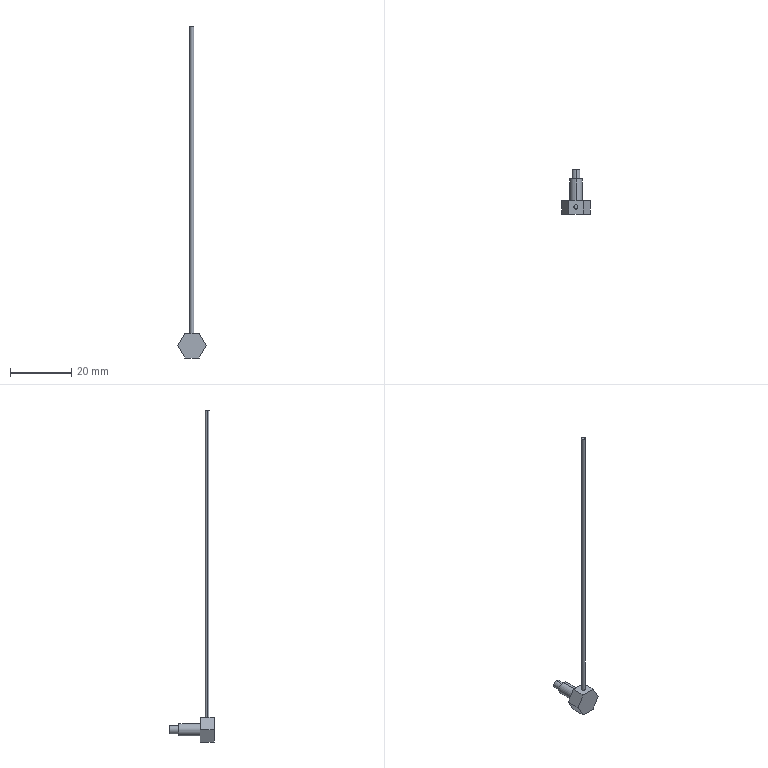Part | SolidWorks | features BaseBody 8 | 1 solid | 17 faces | box 9.238 x 14.5 x 108 mm | volume 486.04 mm3 | plane 11 | cylinder 6 | commonest cylinder face diameters 1.3 x2 2.6 x2 4 x2
STEP:
#1=CARTESIAN_POINT('',(-0.66,0.,100.));
#2=VERTEX_POINT('',#1);
#3=CARTESIAN_POINT('',(0.64,0.,100.));
#4=VERTEX_POINT('',#3);
#5=CARTESIAN_POINT('',(-0.01,0.,100.));
#6=DIRECTION('',(0.,0.,-1.));
#7=DIRECTION('',(-1.,0.,0.));
#8=AXIS2_PLACEMENT_3D('',#5,#6,#7);
#9=CIRCLE('',#8,0.65);
#10=EDGE_CURVE('',#2,#4,#9,.T.);
#11=ORIENTED_EDGE('',*,*,#10,.T.);
#12=CARTESIAN_POINT('',(0.64,0.,0.));
#13=VERTEX_POINT('',#12);
#14=CARTESIAN_POINT('',(0.64,0.,100.));
#15=DIRECTION('',(0.,0.,-1.));
#16=VECTOR('',#15,1000.);
#17=LINE('',#14,#16);
#18=EDGE_CURVE('',#4,#13,#17,.T.);
#19=ORIENTED_EDGE('',*,*,#18,.T.);
#20=CARTESIAN_POINT('',(-0.66,0.,0.));
#21=VERTEX_POINT('',#20);
#22=CARTESIAN_POINT('',(-0.01,0.,0.));
#23=DIRECTION('',(0.,0.,1.));
#24=DIRECTION('',(-1.,0.,0.));
#25=AXIS2_PLACEMENT_3D('',#22,#23,#24);
#26=CIRCLE('',#25,0.65);
#27=EDGE_CURVE('',#13,#21,#26,.T.);
#28=ORIENTED_EDGE('',*,*,#27,.T.);
#29=CARTESIAN_POINT('',(-0.66,0.,100.));
#30=DIRECTION('',(0.,0.,-1.));
#31=VECTOR('',#30,1000.);
#32=LINE('',#29,#31);
#33=EDGE_CURVE('',#2,#21,#32,.T.);
#34=ORIENTED_EDGE('',*,*,#33,.F.);
#35=EDGE_LOOP('',(#11,#19,#28,#34));
#36=FACE_OUTER_BOUND('',#35,.T.);
#37=CARTESIAN_POINT('',(-0.01,0.,100.));
#38=DIRECTION('',(0.,0.,-1.));
#39=DIRECTION('',(-1.,0.,0.));
#40=AXIS2_PLACEMENT_3D('',#37,#38,#39);
#41=CYLINDRICAL_SURFACE('',#40,0.65);
#42=ADVANCED_FACE('',(#36),#41,.T.);
#43=CARTESIAN_POINT('',(0.,9.25,-6.));
#44=VERTEX_POINT('',#43);
#45=CARTESIAN_POINT('',(0.,9.25,-2.));
#46=VERTEX_POINT('',#45);
#47=CARTESIAN_POINT('',(0.,9.25,-4.));
#48=DIRECTION('',(0.,-1.,0.));
#49=DIRECTION('',(0.,0.,-1.));
#50=AXIS2_PLACEMENT_3D('',#47,#48,#49);
#51=CIRCLE('',#50,2.);
#52=EDGE_CURVE('',#44,#46,#51,.T.);
#53=ORIENTED_EDGE('',*,*,#52,.T.);
#54=CARTESIAN_POINT('',(0.,2.25,-2.));
#55=VERTEX_POINT('',#54);
#56=CARTESIAN_POINT('',(0.,9.25,-2.));
#57=DIRECTION('',(0.,-1.,0.));
#58=VECTOR('',#57,1000.);
#59=LINE('',#56,#58);
#60=EDGE_CURVE('',#46,#55,#59,.T.);
#61=ORIENTED_EDGE('',*,*,#60,.T.);
#62=CARTESIAN_POINT('',(0.,2.25,-6.));
#63=VERTEX_POINT('',#62);
#64=CARTESIAN_POINT('',(0.,2.25,-4.));
#65=DIRECTION('',(0.,1.,0.));
#66=DIRECTION('',(0.,0.,-1.));
#67=AXIS2_PLACEMENT_3D('',#64,#65,#66);
#68=CIRCLE('',#67,2.);
#69=EDGE_CURVE('',#55,#63,#68,.T.);
#70=ORIENTED_EDGE('',*,*,#69,.T.);
#71=CARTESIAN_POINT('',(0.,9.25,-6.));
#72=DIRECTION('',(0.,-1.,0.));
#73=VECTOR('',#72,1000.);
#74=LINE('',#71,#73);
#75=EDGE_CURVE('',#44,#63,#74,.T.);
#76=ORIENTED_EDGE('',*,*,#75,.F.);
#77=EDGE_LOOP('',(#53,#61,#70,#76));
#78=FACE_OUTER_BOUND('',#77,.T.);
#79=CARTESIAN_POINT('',(0.,9.25,-4.));
#80=DIRECTION('',(0.,-1.,0.));
#81=DIRECTION('',(0.,0.,-1.));
#82=AXIS2_PLACEMENT_3D('',#79,#80,#81);
#83=CYLINDRICAL_SURFACE('',#82,2.);
#84=ADVANCED_FACE('',(#78),#83,.T.);
#85=CARTESIAN_POINT('',(0.,12.25,-5.3));
#86=VERTEX_POINT('',#85);
#87=CARTESIAN_POINT('',(0.,12.25,-2.7));
#88=VERTEX_POINT('',#87);
#89=CARTESIAN_POINT('',(0.,12.25,-4.));
#90=DIRECTION('',(0.,-1.,0.));
#91=DIRECTION('',(0.,0.,-1.));
#92=AXIS2_PLACEMENT_3D('',#89,#90,#91);
#93=CIRCLE('',#92,1.3);
#94=EDGE_CURVE('',#86,#88,#93,.T.);
#95=ORIENTED_EDGE('',*,*,#94,.T.);
#96=CARTESIAN_POINT('',(0.,9.25,-2.7));
#97=VERTEX_POINT('',#96);
#98=CARTESIAN_POINT('',(0.,12.25,-2.7));
#99=DIRECTION('',(0.,-1.,0.));
#100=VECTOR('',#99,1000.);
#101=LINE('',#98,#100);
#102=EDGE_CURVE('',#88,#97,#101,.T.);
#103=ORIENTED_EDGE('',*,*,#102,.T.);
#104=CARTESIAN_POINT('',(0.,9.25,-5.3));
#105=VERTEX_POINT('',#104);
#106=CARTESIAN_POINT('',(0.,9.25,-4.));
#107=DIRECTION('',(0.,-1.,0.));
#108=DIRECTION('',(0.,0.,-1.));
#109=AXIS2_PLACEMENT_3D('',#106,#107,#108);
#110=CIRCLE('',#109,1.3);
#111=EDGE_CURVE('',#105,#97,#110,.T.);
#112=ORIENTED_EDGE('',*,*,#111,.F.);
#113=CARTESIAN_POINT('',(0.,12.25,-5.3));
#114=DIRECTION('',(0.,-1.,0.));
#115=VECTOR('',#114,1000.);
#116=LINE('',#113,#115);
#117=EDGE_CURVE('',#86,#105,#116,.T.);
#118=ORIENTED_EDGE('',*,*,#117,.F.);
#119=EDGE_LOOP('',(#95,#103,#112,#118));
#120=FACE_OUTER_BOUND('',#119,.T.);
#121=CARTESIAN_POINT('',(0.,12.25,-4.));
#122=DIRECTION('',(0.,-1.,0.));
#123=DIRECTION('',(0.,0.,-1.));
#124=AXIS2_PLACEMENT_3D('',#121,#122,#123);
#125=CYLINDRICAL_SURFACE('',#124,1.3);
#126=ADVANCED_FACE('',(#120),#125,.T.);
#127=ORIENTED_EDGE('',*,*,#18,.F.);
#128=CARTESIAN_POINT('',(-0.01,0.,100.));
#129=DIRECTION('',(0.,0.,-1.));
#130=DIRECTION('',(-1.,0.,0.));
#131=AXIS2_PLACEMENT_3D('',#128,#129,#130);
#132=CIRCLE('',#131,0.65);
#133=EDGE_CURVE('',#4,#2,#132,.T.);
#134=ORIENTED_EDGE('',*,*,#133,.T.);
#135=ORIENTED_EDGE('',*,*,#33,.T.);
#136=CARTESIAN_POINT('',(-0.01,0.,0.));
#137=DIRECTION('',(0.,0.,1.));
#138=DIRECTION('',(-1.,0.,0.));
#139=AXIS2_PLACEMENT_3D('',#136,#137,#138);
#140=CIRCLE('',#139,0.65);
#141=EDGE_CURVE('',#21,#13,#140,.T.);
#142=ORIENTED_EDGE('',*,*,#141,.T.);
#143=EDGE_LOOP('',(#127,#134,#135,#142));
#144=FACE_OUTER_BOUND('',#143,.T.);
#145=CARTESIAN_POINT('',(-0.01,0.,100.));
#146=DIRECTION('',(0.,0.,-1.));
#147=DIRECTION('',(-1.,0.,0.));
#148=AXIS2_PLACEMENT_3D('',#145,#146,#147);
#149=CYLINDRICAL_SURFACE('',#148,0.65);
#150=ADVANCED_FACE('',(#144),#149,.T.);
#151=ORIENTED_EDGE('',*,*,#141,.F.);
#152=ORIENTED_EDGE('',*,*,#27,.F.);
#153=EDGE_LOOP('',(#151,#152));
#154=FACE_BOUND('',#153,.T.);
#155=CARTESIAN_POINT('',(-2.309,-2.25,0.));
#156=VERTEX_POINT('',#155);
#157=CARTESIAN_POINT('',(-2.309,2.25,0.));
#158=VERTEX_POINT('',#157);
#159=CARTESIAN_POINT('',(-2.309,-2.25,0.));
#160=DIRECTION('',(0.,1.,0.));
#161=VECTOR('',#160,1000.);
#162=LINE('',#159,#161);
#163=EDGE_CURVE('',#156,#158,#162,.T.);
#164=ORIENTED_EDGE('',*,*,#163,.F.);
#165=CARTESIAN_POINT('',(2.309,-2.25,0.));
#166=VERTEX_POINT('',#165);
#167=CARTESIAN_POINT('',(-2.309,-2.25,0.));
#168=DIRECTION('',(-1.,0.,0.));
#169=VECTOR('',#168,1000.);
#170=LINE('',#167,#169);
#171=EDGE_CURVE('',#166,#156,#170,.T.);
#172=ORIENTED_EDGE('',*,*,#171,.F.);
#173=CARTESIAN_POINT('',(2.309,2.25,0.));
#174=VERTEX_POINT('',#173);
#175=CARTESIAN_POINT('',(2.309,-2.25,0.));
#176=DIRECTION('',(0.,-1.,0.));
#177=VECTOR('',#176,1000.);
#178=LINE('',#175,#177);
#179=EDGE_CURVE('',#174,#166,#178,.T.);
#180=ORIENTED_EDGE('',*,*,#179,.F.);
#181=CARTESIAN_POINT('',(-2.309,2.25,0.));
#182=DIRECTION('',(1.,0.,0.));
#183=VECTOR('',#182,1000.);
#184=LINE('',#181,#183);
#185=EDGE_CURVE('',#158,#174,#184,.T.);
#186=ORIENTED_EDGE('',*,*,#185,.F.);
#187=EDGE_LOOP('',(#164,#172,#180,#186));
#188=FACE_OUTER_BOUND('',#187,.T.);
#189=CARTESIAN_POINT('',(-2.309,-2.25,0.));
#190=DIRECTION('',(0.,0.,-1.));
#191=DIRECTION('',(-1.,0.,0.));
#192=AXIS2_PLACEMENT_3D('',#189,#190,#191);
#193=PLANE('',#192);
#194=ADVANCED_FACE('',(#154,#188),#193,.F.);
#195=ORIENTED_EDGE('',*,*,#10,.F.);
#196=ORIENTED_EDGE('',*,*,#133,.F.);
#197=EDGE_LOOP('',(#195,#196));
#198=FACE_OUTER_BOUND('',#197,.T.);
#199=CARTESIAN_POINT('',(-0.01,0.,100.));
#200=DIRECTION('',(0.,0.,1.));
#201=DIRECTION('',(1.,0.,0.));
#202=AXIS2_PLACEMENT_3D('',#199,#200,#201);
#203=PLANE('',#202);
#204=ADVANCED_FACE('',(#198),#203,.T.);
#205=CARTESIAN_POINT('',(0.,2.25,-4.));
#206=DIRECTION('',(0.,1.,0.));
#207=DIRECTION('',(0.,0.,-1.));
#208=AXIS2_PLACEMENT_3D('',#205,#206,#207);
#209=CIRCLE('',#208,2.);
#210=EDGE_CURVE('',#63,#55,#209,.T.);
#211=ORIENTED_EDGE('',*,*,#210,.F.);
#212=ORIENTED_EDGE('',*,*,#69,.F.);
#213=EDGE_LOOP('',(#211,#212));
#214=FACE_BOUND('',#213,.T.);
#215=ORIENTED_EDGE('',*,*,#185,.T.);
#216=CARTESIAN_POINT('',(4.619,2.25,-4.));
#217=VERTEX_POINT('',#216);
#218=CARTESIAN_POINT('',(4.619,2.25,-4.));
#219=DIRECTION('',(-0.5,0.,0.866));
#220=VECTOR('',#219,1000.);
#221=LINE('',#218,#220);
#222=EDGE_CURVE('',#217,#174,#221,.T.);
#223=ORIENTED_EDGE('',*,*,#222,.F.);
#224=CARTESIAN_POINT('',(2.309,2.25,-8.));
#225=VERTEX_POINT('',#224);
#226=CARTESIAN_POINT('',(2.309,2.25,-8.));
#227=DIRECTION('',(0.5,0.,0.866));
#228=VECTOR('',#227,1000.);
#229=LINE('',#226,#228);
#230=EDGE_CURVE('',#225,#217,#229,.T.);
#231=ORIENTED_EDGE('',*,*,#230,.F.);
#232=CARTESIAN_POINT('',(-2.309,2.25,-8.));
#233=VERTEX_POINT('',#232);
#234=CARTESIAN_POINT('',(-2.309,2.25,-8.));
#235=DIRECTION('',(1.,0.,0.));
#236=VECTOR('',#235,1000.);
#237=LINE('',#234,#236);
#238=EDGE_CURVE('',#233,#225,#237,.T.);
#239=ORIENTED_EDGE('',*,*,#238,.F.);
#240=CARTESIAN_POINT('',(-4.619,2.25,-4.));
#241=VERTEX_POINT('',#240);
#242=CARTESIAN_POINT('',(-4.619,2.25,-4.));
#243=DIRECTION('',(0.5,0.,-0.866));
#244=VECTOR('',#243,1000.);
#245=LINE('',#242,#244);
#246=EDGE_CURVE('',#241,#233,#245,.T.);
#247=ORIENTED_EDGE('',*,*,#246,.F.);
#248=CARTESIAN_POINT('',(-2.309,2.25,0.));
#249=DIRECTION('',(-0.5,0.,-0.866));
#250=VECTOR('',#249,1000.);
#251=LINE('',#248,#250);
#252=EDGE_CURVE('',#158,#241,#251,.T.);
#253=ORIENTED_EDGE('',*,*,#252,.F.);
#254=EDGE_LOOP('',(#215,#223,#231,#239,#247,#253));
#255=FACE_OUTER_BOUND('',#254,.T.);
#256=CARTESIAN_POINT('',(-2.309,2.25,0.));
#257=DIRECTION('',(0.,-1.,0.));
#258=DIRECTION('',(0.,0.,-1.));
#259=AXIS2_PLACEMENT_3D('',#256,#257,#258);
#260=PLANE('',#259);
#261=ADVANCED_FACE('',(#214,#255),#260,.F.);
#262=CARTESIAN_POINT('',(-4.619,-2.25,-4.));
#263=VERTEX_POINT('',#262);
#264=CARTESIAN_POINT('',(-4.619,-2.25,-4.));
#265=DIRECTION('',(0.,1.,0.));
#266=VECTOR('',#265,1000.);
#267=LINE('',#264,#266);
#268=EDGE_CURVE('',#263,#241,#267,.T.);
#269=ORIENTED_EDGE('',*,*,#268,.F.);
#270=CARTESIAN_POINT('',(-4.619,-2.25,-4.));
#271=DIRECTION('',(-0.5,0.,-0.866));
#272=VECTOR('',#271,1000.);
#273=LINE('',#270,#272);
#274=EDGE_CURVE('',#156,#263,#273,.T.);
#275=ORIENTED_EDGE('',*,*,#274,.F.);
#276=ORIENTED_EDGE('',*,*,#163,.T.);
#277=ORIENTED_EDGE('',*,*,#252,.T.);
#278=EDGE_LOOP('',(#269,#275,#276,#277));
#279=FACE_OUTER_BOUND('',#278,.T.);
#280=CARTESIAN_POINT('',(-4.619,-2.25,-4.));
#281=DIRECTION('',(0.866,0.,-0.5));
#282=DIRECTION('',(-0.5,0.,-0.866));
#283=AXIS2_PLACEMENT_3D('',#280,#281,#282);
#284=PLANE('',#283);
#285=ADVANCED_FACE('',(#279),#284,.F.);
#286=CARTESIAN_POINT('',(4.619,-2.25,-4.));
#287=VERTEX_POINT('',#286);
#288=CARTESIAN_POINT('',(4.619,-2.25,-4.));
#289=DIRECTION('',(-0.5,0.,0.866));
#290=VECTOR('',#289,1000.);
#291=LINE('',#288,#290);
#292=EDGE_CURVE('',#287,#166,#291,.T.);
#293=ORIENTED_EDGE('',*,*,#292,.T.);
#294=ORIENTED_EDGE('',*,*,#171,.T.);
#295=ORIENTED_EDGE('',*,*,#274,.T.);
#296=CARTESIAN_POINT('',(-2.309,-2.25,-8.));
#297=VERTEX_POINT('',#296);
#298=CARTESIAN_POINT('',(-4.619,-2.25,-4.));
#299=DIRECTION('',(0.5,0.,-0.866));
#300=VECTOR('',#299,1000.);
#301=LINE('',#298,#300);
#302=EDGE_CURVE('',#263,#297,#301,.T.);
#303=ORIENTED_EDGE('',*,*,#302,.T.);
#304=CARTESIAN_POINT('',(2.309,-2.25,-8.));
#305=VERTEX_POINT('',#304);
#306=CARTESIAN_POINT('',(-2.309,-2.25,-8.));
#307=DIRECTION('',(1.,0.,0.));
#308=VECTOR('',#307,1000.);
#309=LINE('',#306,#308);
#310=EDGE_CURVE('',#297,#305,#309,.T.);
#311=ORIENTED_EDGE('',*,*,#310,.T.);
#312=CARTESIAN_POINT('',(2.309,-2.25,-8.));
#313=DIRECTION('',(0.5,0.,0.866));
#314=VECTOR('',#313,1000.);
#315=LINE('',#312,#314);
#316=EDGE_CURVE('',#305,#287,#315,.T.);
#317=ORIENTED_EDGE('',*,*,#316,.T.);
#318=EDGE_LOOP('',(#293,#294,#295,#303,#311,#317));
#319=FACE_OUTER_BOUND('',#318,.T.);
#320=CARTESIAN_POINT('',(-2.309,-2.25,0.));
#321=DIRECTION('',(0.,-1.,0.));
#322=DIRECTION('',(0.,0.,-1.));
#323=AXIS2_PLACEMENT_3D('',#320,#321,#322);
#324=PLANE('',#323);
#325=ADVANCED_FACE('',(#319),#324,.T.);
#326=ORIENTED_EDGE('',*,*,#179,.T.);
#327=ORIENTED_EDGE('',*,*,#292,.F.);
#328=CARTESIAN_POINT('',(4.619,-2.25,-4.));
#329=DIRECTION('',(0.,-1.,0.));
#330=VECTOR('',#329,1000.);
#331=LINE('',#328,#330);
#332=EDGE_CURVE('',#217,#287,#331,.T.);
#333=ORIENTED_EDGE('',*,*,#332,.F.);
#334=ORIENTED_EDGE('',*,*,#222,.T.);
#335=EDGE_LOOP('',(#326,#327,#333,#334));
#336=FACE_OUTER_BOUND('',#335,.T.);
#337=CARTESIAN_POINT('',(2.309,-2.25,0.));
#338=DIRECTION('',(-0.866,0.,-0.5));
#339=DIRECTION('',(-0.5,0.,0.866));
#340=AXIS2_PLACEMENT_3D('',#337,#338,#339);
#341=PLANE('',#340);
#342=ADVANCED_FACE('',(#336),#341,.F.);
#343=ORIENTED_EDGE('',*,*,#60,.F.);
#344=CARTESIAN_POINT('',(0.,9.25,-4.));
#345=DIRECTION('',(0.,-1.,0.));
#346=DIRECTION('',(0.,0.,-1.));
#347=AXIS2_PLACEMENT_3D('',#344,#345,#346);
#348=CIRCLE('',#347,2.);
#349=EDGE_CURVE('',#46,#44,#348,.T.);
#350=ORIENTED_EDGE('',*,*,#349,.T.);
#351=ORIENTED_EDGE('',*,*,#75,.T.);
#352=ORIENTED_EDGE('',*,*,#210,.T.);
#353=EDGE_LOOP('',(#343,#350,#351,#352));
#354=FACE_OUTER_BOUND('',#353,.T.);
#355=CARTESIAN_POINT('',(0.,9.25,-4.));
#356=DIRECTION('',(0.,-1.,0.));
#357=DIRECTION('',(0.,0.,-1.));
#358=AXIS2_PLACEMENT_3D('',#355,#356,#357);
#359=CYLINDRICAL_SURFACE('',#358,2.);
#360=ADVANCED_FACE('',(#354),#359,.T.);
#361=ORIENTED_EDGE('',*,*,#332,.T.);
#362=ORIENTED_EDGE('',*,*,#316,.F.);
#363=CARTESIAN_POINT('',(2.309,-2.25,-8.));
#364=DIRECTION('',(0.,-1.,0.));
#365=VECTOR('',#364,1000.);
#366=LINE('',#363,#365);
#367=EDGE_CURVE('',#225,#305,#366,.T.);
#368=ORIENTED_EDGE('',*,*,#367,.F.);
#369=ORIENTED_EDGE('',*,*,#230,.T.);
#370=EDGE_LOOP('',(#361,#362,#368,#369));
#371=FACE_OUTER_BOUND('',#370,.T.);
#372=CARTESIAN_POINT('',(4.619,-2.25,-4.));
#373=DIRECTION('',(-0.866,0.,0.5));
#374=DIRECTION('',(0.5,0.,0.866));
#375=AXIS2_PLACEMENT_3D('',#372,#373,#374);
#376=PLANE('',#375);
#377=ADVANCED_FACE('',(#371),#376,.F.);
#378=ORIENTED_EDGE('',*,*,#367,.T.);
#379=ORIENTED_EDGE('',*,*,#310,.F.);
#380=CARTESIAN_POINT('',(-2.309,-2.25,-8.));
#381=DIRECTION('',(0.,-1.,0.));
#382=VECTOR('',#381,1000.);
#383=LINE('',#380,#382);
#384=EDGE_CURVE('',#233,#297,#383,.T.);
#385=ORIENTED_EDGE('',*,*,#384,.F.);
#386=ORIENTED_EDGE('',*,*,#238,.T.);
#387=EDGE_LOOP('',(#378,#379,#385,#386));
#388=FACE_OUTER_BOUND('',#387,.T.);
#389=CARTESIAN_POINT('',(2.309,-2.25,-8.));
#390=DIRECTION('',(0.,0.,1.));
#391=DIRECTION('',(1.,0.,0.));
#392=AXIS2_PLACEMENT_3D('',#389,#390,#391);
#393=PLANE('',#392);
#394=ADVANCED_FACE('',(#388),#393,.F.);
#395=ORIENTED_EDGE('',*,*,#384,.T.);
#396=ORIENTED_EDGE('',*,*,#302,.F.);
#397=ORIENTED_EDGE('',*,*,#268,.T.);
#398=ORIENTED_EDGE('',*,*,#246,.T.);
#399=EDGE_LOOP('',(#395,#396,#397,#398));
#400=FACE_OUTER_BOUND('',#399,.T.);
#401=CARTESIAN_POINT('',(-2.309,-2.25,-8.));
#402=DIRECTION('',(0.866,0.,0.5));
#403=DIRECTION('',(0.5,0.,-0.866));
#404=AXIS2_PLACEMENT_3D('',#401,#402,#403);
#405=PLANE('',#404);
#406=ADVANCED_FACE('',(#400),#405,.F.);
#407=ORIENTED_EDGE('',*,*,#111,.T.);
#408=CARTESIAN_POINT('',(0.,9.25,-4.));
#409=DIRECTION('',(0.,-1.,0.));
#410=DIRECTION('',(0.,0.,-1.));
#411=AXIS2_PLACEMENT_3D('',#408,#409,#410);
#412=CIRCLE('',#411,1.3);
#413=EDGE_CURVE('',#97,#105,#412,.T.);
#414=ORIENTED_EDGE('',*,*,#413,.T.);
#415=EDGE_LOOP('',(#407,#414));
#416=FACE_BOUND('',#415,.T.);
#417=ORIENTED_EDGE('',*,*,#52,.F.);
#418=ORIENTED_EDGE('',*,*,#349,.F.);
#419=EDGE_LOOP('',(#417,#418));
#420=FACE_OUTER_BOUND('',#419,.T.);
#421=CARTESIAN_POINT('',(0.,9.25,-4.));
#422=DIRECTION('',(0.,1.,0.));
#423=DIRECTION('',(0.,0.,1.));
#424=AXIS2_PLACEMENT_3D('',#421,#422,#423);
#425=PLANE('',#424);
#426=ADVANCED_FACE('',(#416,#420),#425,.T.);
#427=ORIENTED_EDGE('',*,*,#102,.F.);
#428=CARTESIAN_POINT('',(0.,12.25,-4.));
#429=DIRECTION('',(0.,-1.,0.));
#430=DIRECTION('',(0.,0.,-1.));
#431=AXIS2_PLACEMENT_3D('',#428,#429,#430);
#432=CIRCLE('',#431,1.3);
#433=EDGE_CURVE('',#88,#86,#432,.T.);
#434=ORIENTED_EDGE('',*,*,#433,.T.);
#435=ORIENTED_EDGE('',*,*,#117,.T.);
#436=ORIENTED_EDGE('',*,*,#413,.F.);
#437=EDGE_LOOP('',(#427,#434,#435,#436));
#438=FACE_OUTER_BOUND('',#437,.T.);
#439=CARTESIAN_POINT('',(0.,12.25,-4.));
#440=DIRECTION('',(0.,-1.,0.));
#441=DIRECTION('',(0.,0.,-1.));
#442=AXIS2_PLACEMENT_3D('',#439,#440,#441);
#443=CYLINDRICAL_SURFACE('',#442,1.3);
#444=ADVANCED_FACE('',(#438),#443,.T.);
#445=ORIENTED_EDGE('',*,*,#94,.F.);
#446=ORIENTED_EDGE('',*,*,#433,.F.);
#447=EDGE_LOOP('',(#445,#446));
#448=FACE_OUTER_BOUND('',#447,.T.);
#449=CARTESIAN_POINT('',(0.,12.25,-4.));
#450=DIRECTION('',(0.,-1.,0.));
#451=DIRECTION('',(0.,0.,-1.));
#452=AXIS2_PLACEMENT_3D('',#449,#450,#451);
#453=PLANE('',#452);
#454=ADVANCED_FACE('',(#448),#453,.F.);
#455=CLOSED_SHELL('',(#42,#84,#126,#150,#194,#204,#261,#285,#325,#342,#360,#377,#394,#406,#426,#444,#454));
#456=MANIFOLD_SOLID_BREP('',#455);
#457=CARTESIAN_POINT('',(0.,0.,0.));
#458=DIRECTION('',(0.,0.,1.));
#459=DIRECTION('',(1.,0.,0.));
#460=AXIS2_PLACEMENT_3D('',#457,#458,#459);
#461=(LENGTH_UNIT()NAMED_UNIT(*)SI_UNIT(.MILLI.,.METRE.));
#462=UNCERTAINTY_MEASURE_WITH_UNIT(LENGTH_MEASURE(0.00001),#461,'','');
#463=(NAMED_UNIT(*)PLANE_ANGLE_UNIT()SI_UNIT($,.RADIAN.));
#464=(NAMED_UNIT(*)SI_UNIT($,.STERADIAN.)SOLID_ANGLE_UNIT());
#465=(GEOMETRIC_REPRESENTATION_CONTEXT(3)GLOBAL_UNCERTAINTY_ASSIGNED_CONTEXT((#462))GLOBAL_UNIT_ASSIGNED_CONTEXT((#461,#463,#464))REPRESENTATION_CONTEXT('',''));
#466=ADVANCED_BREP_SHAPE_REPRESENTATION('',(#456,#460),#465);